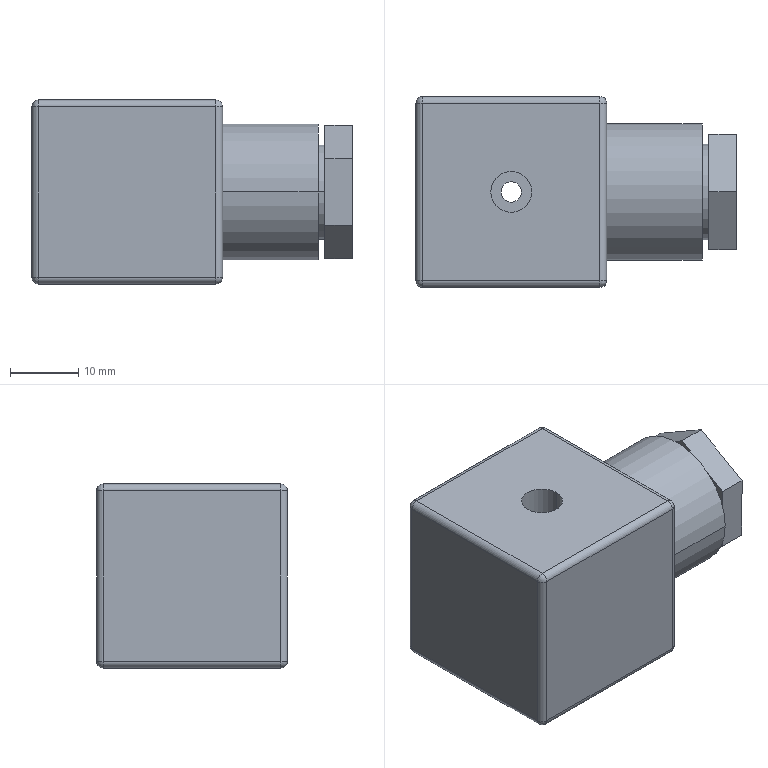Part | SolidWorks | features ICE 4, Cut 3, BossThin 1, Extrusion 1, Fillet 1 | 1 solid | 75 faces | box 47 x 28 x 27 mm | volume 22698 mm3 | plane 45 | cylinder 22 | sphere 8 | commonest cylinder face diameters 2 x12 3 x2 6 x2 12 x2 14 x2 20 x2